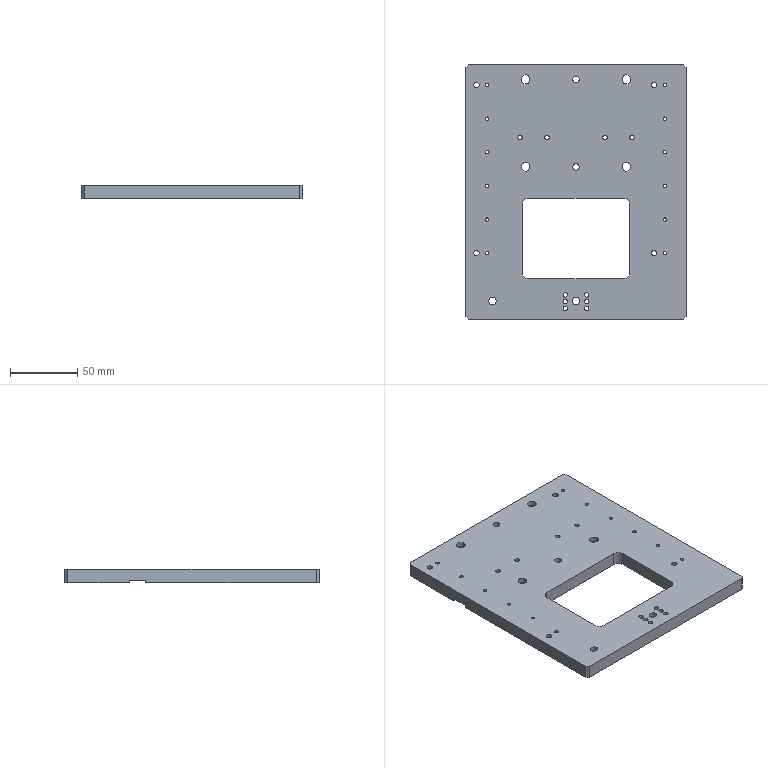CAM job | NX | 3-axis milling, drilling | part box 164 x 189 x 10 mm | stock box 169 x 194 x 10 mm
Tools:
number,name,description,diameter,corner_radius,flute_length,length,flutes
6,D6,平底铣刀-粗,6.0,0.0,25.0,75.0,2
9,D10,平底铣刀-粗,10.0,0.0,35.0,75.0,2
17,D2-J,平底铣刀-精,2.0,0.0,50.0,75.0,2
11,D3-J,平底铣刀-精,3.0,0.0,50.0,75.0,2
7,D6-J,平底铣刀-精,6.0,0.0,25.0,75.0,2
2,D6倒角刀,倒角刀,6.0,0.0,3.0,25.0,2
12,ZT2.6,钻头,2.6,0.0,35.0,50.0,2
13,ZT3.4,钻头,3.4,0.0,35.0,50.0,2
20,ZT5.5,钻头,5.5,0.0,35.0,50.0,2
23,钻头6.6,Drilling Tool,6.6,0.0,35.0,50.0,2
18,ZT3.9,Drilling Tool,3.9,0.0,35.0,50.0,2
19,ZT4.9,Drilling Tool,4.9,0.0,35.0,50.0,2
Operations:
program,operation,operation_type,tool,method,geometry_group,spindle_rpm,surface_speed,feed_per_tooth,feed_cut,feed_plunge,cut_length_mm,path_length_mm,cut_time_min,machine_time_min
B,C0.3封闭铣廓倒角6X45L_COPY,PlanarMilling,D6倒角刀,爬面_倒角-切深0-步距G,W-B,7000.0,131.0,0.1071,1500.0,100.0,1304.291,3472.148,0.8695,1.086
B,钻倒角_5,Operation,D6倒角刀,METHOD,W-B,8000.0,150.796,0.0625,1000.0,0.0,57.0,630.828,0.057,0.1144
B,钻倒角_6,Operation,D6倒角刀,METHOD,W-B,8000.0,150.796,0.0625,1000.0,0.0,52.0,475.893,0.052,0.0944
B,钻倒角_7,Operation,D6倒角刀,METHOD,W-B,8000.0,150.796,0.0625,1000.0,0.0,21.2,533.506,0.0212,0.0724
B,钻倒角_8,Operation,D6倒角刀,METHOD,W-B,8000.0,150.796,0.0625,1000.0,0.0,11.6,191.269,0.0116,0.0296
B,铣倒角_3,PlanarMilling,D6倒角刀,METHOD,W-B,8000.0,150.796,0.075,1200.0,100.0,35.589,301.203,0.0297,0.0562
B,铣倒角_4,PlanarMilling,D6倒角刀,METHOD,W-B,8000.0,150.796,0.075,1200.0,100.0,81.784,694.015,0.0682,0.1294
A,打点,Operation,D6倒角刀,METHOD,W-A,3000.0,56.549,0.0333,200.0,0.0,5.0,136.008,0.025,0.0381
A,打点_2,Operation,D6倒角刀,METHOD,W-A,3000.0,56.549,0.0333,200.0,0.0,24.0,501.204,0.12,0.1677
A,打点_3,Operation,D6倒角刀,METHOD,W-A,3000.0,56.549,0.0333,200.0,0.0,50.0,754.222,0.25,0.3204
A,打孔,Operation,ZT2.6,METHOD,W-A,3800.0,29.845,0.0105,80.0,0.0,126.0,705.204,1.575,1.633
A,打孔_2,Operation,ZT3.4,METHOD,W-A,3500.0,36.285,0.0143,100.0,0.0,105.0,520.194,1.05,1.091
A,打孔_3,Operation,ZT3.9,METHOD,W-A,3000.0,35.814,0.02,120.0,0.0,42.0,529.012,0.35,0.3987
A,打孔_4,Operation,ZT4.9,METHOD,W-A,3000.0,45.239,0.025,150.0,0.0,21.0,168.008,0.14,0.1547
A,打孔_5,Operation,ZT5.5,METHOD,W-A,2600.0,44.925,0.0231,120.0,0.0,21.0,165.008,0.175,0.1894
A,打孔_6,Operation,钻头6.6,METHOD,W-A,2500.0,51.836,0.03,150.0,0.0,42.0,352.022,0.28,0.311
A,孔粗_1,CylinderMilling,D6,METHOD,W-A,6000.0,113.097,0.1667,2000.0,100.0,424.898,617.098,0.2124,0.2317
A,孔粗_2,CylinderMilling,D6,METHOD,W-A,6000.0,113.097,0.1667,2000.0,100.0,899.191,1368.591,0.4496,0.4965
A,底壁粗_1,VolumeBased25DMillingOperation,D10,METHOD,W-A,6000.0,113.0,0.2083,3500.0,100.0,1495.386,1668.218,0.4273,0.4445
A,框开粗_1,VolumeBased25DMillingOperation,D10,METHOD,W-A,6000.0,188.0,0.25,4000.0,80.0,5024.711,5092.711,1.256,1.263
A,外形粗_2,VolumeBased25DMillingOperation,D10,METHOD,W-A,6000.0,188.0,0.25,4000.0,80.0,15402.02,15470.02,3.85,3.857
A,框半精_1,VolumeBased25DMillingOperation,D6-J,METHOD,W-A,6000.0,113.0,0.0833,1000.0,100.0,258.608,336.608,0.2586,0.2664
A,框精_1,VolumeBased25DMillingOperation,D6-J,METHOD,W-A,6000.0,113.0,0.0833,1000.0,100.0,257.722,336.322,0.2577,0.2656
A,孔侧_1,CylinderMilling,D6-J,METHOD,W-A,6000.0,113.097,0.05,600.0,100.0,35.113,238.713,0.0585,0.0789
A,孔侧_2,CylinderMilling,D6-J,METHOD,W-A,6000.0,113.097,0.0667,800.0,100.0,86.767,582.967,0.1085,0.1581
A,底精_1,VolumeBased25DMillingOperation,D6-J,METHOD,W-A,6000.0,113.0,0.2083,1200.0,100.0,674.3,737.3,0.5619,0.5682
A,底侧精_3,VolumeBased25DMillingOperation,D6-J,METHOD,W-A,6000.0,113.0,0.0833,1000.0,100.0,350.323,413.323,0.3503,0.3566
A,底壁铣螺旋精光-中_COPY_COPY_COPY_1,VolumeBased25DMillingOperation,D2-J,螺旋精光-切深K-步距G,W-A,8000.0,50.266,0.0187,300.0,100.0,921.168,1851.446,3.071,3.164
A,底壁铣螺旋精光-中_COPY_COPY_COPY_1_COPY,VolumeBased25DMillingOperation,D3-J,螺旋精光-切深K-步距G,W-A,8000.0,50.266,0.0187,300.0,100.0,589.628,1411.184,1.965,2.048
A,仅选体,SurfaceContour,D6倒角刀,METHOD,W-A,6000.0,113.0,0.125,1200.0,100.0,1348.111,1975.39,1.123,1.186
A,钻倒角_1,Operation,D6倒角刀,METHOD,W-A,5000.0,94.248,0.015,150.0,0.0,57.0,590.828,0.38,0.4334
A,钻倒角_2,Operation,D6倒角刀,METHOD,W-A,5000.0,94.248,0.015,150.0,0.0,52.0,437.959,0.3467,0.3853
A,钻倒角_3,Operation,D6倒角刀,METHOD,W-A,5000.0,94.248,0.015,150.0,0.0,21.2,493.506,0.1413,0.1886
A,钻倒角_4,Operation,D6倒角刀,METHOD,W-A,5000.0,94.248,0.015,150.0,0.0,11.6,151.269,0.0773,0.0913
A,铣倒角_1,PlanarMilling,D6倒角刀,METHOD,W-A,6000.0,113.097,0.05,600.0,100.0,65.178,253.347,0.1086,0.1274
A,铣倒角_2,PlanarMilling,D6倒角刀,METHOD,W-A,6000.0,113.097,0.05,600.0,100.0,139.642,596.837,0.2327,0.2785
A,底壁铣螺旋精光-中_COPY_COPY,VolumeBased25DMillingOperation,D2-J,螺旋精光-切深K-步距G,W-A,8000.0,50.266,0.0187,300.0,100.0,579.121,1236.858,1.93,1.996
A,底壁铣螺旋精光-中_COPY_COPY_COPY,VolumeBased25DMillingOperation,D3-J,螺旋精光-切深K-步距G,W-A,8000.0,50.266,0.0187,300.0,100.0,289.56,492.993,0.9652,0.9855
A,外形半精_2,VolumeBased25DMillingOperation,D6-J,METHOD,W-A,6000.0,113.0,0.0833,1000.0,100.0,725.08,803.08,0.7251,0.7329
A,外形精_2,VolumeBased25DMillingOperation,D6-J,METHOD,W-A,6000.0,113.0,0.0833,1000.0,100.0,724.88,803.48,0.7249,0.7327